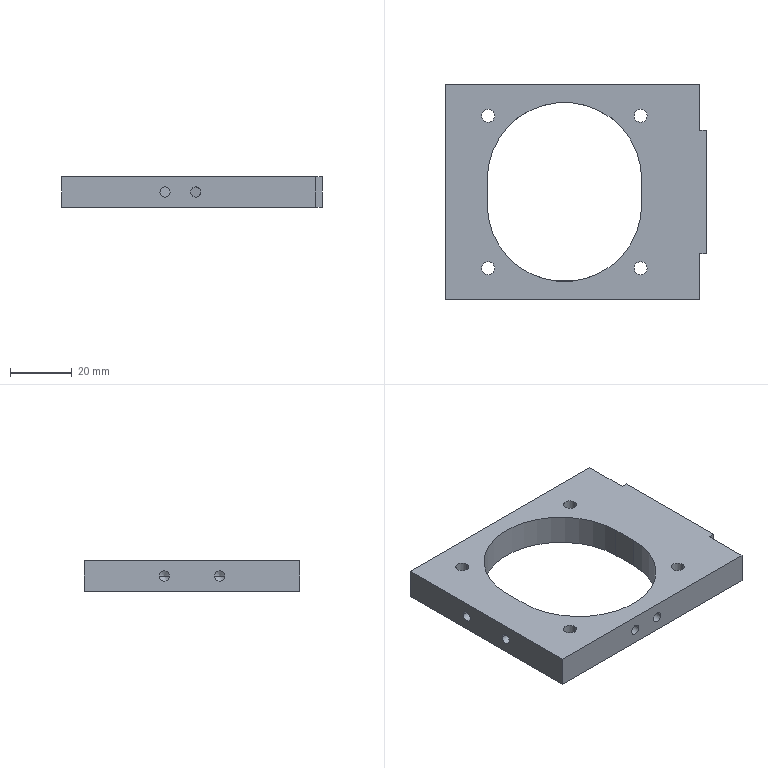CAM job | NX | 3-axis milling, drilling | part box 84.5 x 70 x 10 mm | stock box 90.5 x 74 x 11 mm
Tools:
number,name,description,diameter,corner_radius,flute_length,length,flutes
1,D50,Milling Tool-5 Parameters,50.0,0.0,50.0,75.0,2
2,D6A45,Milling Tool-5 Parameters,6.0,0.0,3.0,3.0,2
14,4.2ZT,Drilling Tool,4.2,0.0,35.0,50.0,2
3,D10,Milling Tool-5 Parameters,10.0,0.0,50.0,75.0,2
4,D10JING,Milling Tool-5 Parameters,10.0,0.0,50.0,75.0,2
Operations:
program,operation,operation_type,tool,method,geometry_group,spindle_rpm,surface_speed,feed_per_tooth,feed_cut,feed_plunge,cut_length_mm,path_length_mm,cut_time_min,machine_time_min
1-87-70-12毛胚,FLOOR_WALL,VolumeBased25DMillingOperation,D50,METHOD,A,6500.0,1286.0,0.0962,1250.0,100.0,487.497,541.497,0.39,0.3954
1-87-70-12毛胚,DRILLING_COPY_1,Operation,D6A45,METHOD,A,3000.0,56.0,0.0333,200.0,0.0,20.4,258.572,0.102,0.1258
1-87-70-12毛胚,DRILLING_COPY_1_COPY_COPY_COPY_COPY,Operation,4.2ZT,METHOD,A,2000.0,20.0,0.0375,150.0,0.0,59.047,335.867,0.3936,0.4213
1-87-70-12毛胚,ADAPTIVE_MILLING,CavityMilling,D10,METHOD,A,7000.0,219.0,0.2143,3000.0,1000.0,5690.154,5890.874,2.395,2.415
1-87-70-12毛胚,ZLEVEL_PROFILE_COPY_COPY_1_COPY_COPY_COPY_1,ZLevelMilling,D10JING,METHOD,A,7000.0,219.0,0.0714,1000.0,100.0,486.404,689.627,0.4864,0.5067
1-87-70-12毛胚,ZLEVEL_PROFILE_COPY_1_COPY_COPY_COPY_COPY_2_COPY,ZLevelMilling,D6A45,METHOD,A,7000.0,131.0,0.0714,1000.0,1000.0,523.522,1135.469,0.5235,0.5847